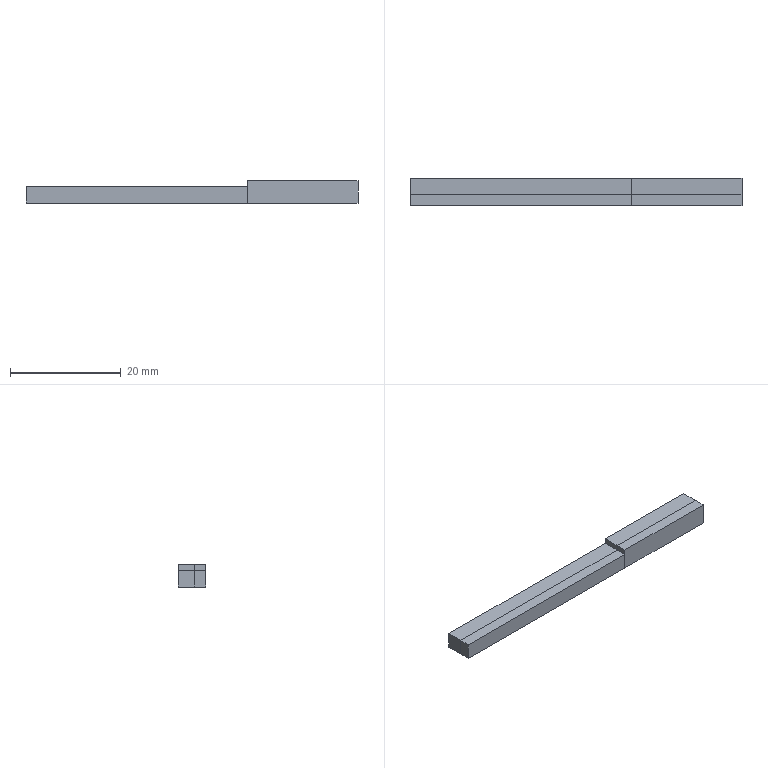Part | SolidWorks | features ICE 3, Extrusion 1 | 4 solids | 24 faces | box 60 x 5 x 4 mm | volume 1000 mm3 | plane 24
STEP:
#1=CARTESIAN_POINT('',(-10.,0.,-2.));
#2=VERTEX_POINT('',#1);
#3=CARTESIAN_POINT('',(-10.,0.,2.));
#4=VERTEX_POINT('',#3);
#5=CARTESIAN_POINT('',(-10.,0.,2.));
#6=DIRECTION('',(0.,0.,1.));
#7=VECTOR('',#6,1000.);
#8=LINE('',#5,#7);
#9=EDGE_CURVE('',#2,#4,#8,.T.);
#10=ORIENTED_EDGE('',*,*,#9,.T.);
#11=CARTESIAN_POINT('',(-10.,2.,2.));
#12=VERTEX_POINT('',#11);
#13=CARTESIAN_POINT('',(-10.,2.,2.));
#14=DIRECTION('',(0.,-1.,0.));
#15=VECTOR('',#14,1000.);
#16=LINE('',#13,#15);
#17=EDGE_CURVE('',#12,#4,#16,.T.);
#18=ORIENTED_EDGE('',*,*,#17,.F.);
#19=CARTESIAN_POINT('',(-10.,2.,-2.));
#20=VERTEX_POINT('',#19);
#21=CARTESIAN_POINT('',(-10.,2.,2.));
#22=DIRECTION('',(0.,0.,1.));
#23=VECTOR('',#22,1000.);
#24=LINE('',#21,#23);
#25=EDGE_CURVE('',#20,#12,#24,.T.);
#26=ORIENTED_EDGE('',*,*,#25,.F.);
#27=CARTESIAN_POINT('',(-10.,2.,-2.));
#28=DIRECTION('',(0.,-1.,0.));
#29=VECTOR('',#28,1000.);
#30=LINE('',#27,#29);
#31=EDGE_CURVE('',#20,#2,#30,.T.);
#32=ORIENTED_EDGE('',*,*,#31,.T.);
#33=EDGE_LOOP('',(#10,#18,#26,#32));
#34=FACE_OUTER_BOUND('',#33,.T.);
#35=CARTESIAN_POINT('',(-10.,2.,2.));
#36=DIRECTION('',(1.,0.,0.));
#37=DIRECTION('',(0.,0.,-1.));
#38=AXIS2_PLACEMENT_3D('',#35,#36,#37);
#39=PLANE('',#38);
#40=ADVANCED_FACE('',(#34),#39,.F.);
#41=CARTESIAN_POINT('',(10.,0.,2.));
#42=VERTEX_POINT('',#41);
#43=CARTESIAN_POINT('',(10.,0.,2.));
#44=DIRECTION('',(1.,0.,0.));
#45=VECTOR('',#44,1000.);
#46=LINE('',#43,#45);
#47=EDGE_CURVE('',#4,#42,#46,.T.);
#48=ORIENTED_EDGE('',*,*,#47,.T.);
#49=CARTESIAN_POINT('',(10.,2.,2.));
#50=VERTEX_POINT('',#49);
#51=CARTESIAN_POINT('',(10.,2.,2.));
#52=DIRECTION('',(0.,-1.,0.));
#53=VECTOR('',#52,1000.);
#54=LINE('',#51,#53);
#55=EDGE_CURVE('',#50,#42,#54,.T.);
#56=ORIENTED_EDGE('',*,*,#55,.F.);
#57=CARTESIAN_POINT('',(10.,2.,2.));
#58=DIRECTION('',(1.,0.,0.));
#59=VECTOR('',#58,1000.);
#60=LINE('',#57,#59);
#61=EDGE_CURVE('',#12,#50,#60,.T.);
#62=ORIENTED_EDGE('',*,*,#61,.F.);
#63=ORIENTED_EDGE('',*,*,#17,.T.);
#64=EDGE_LOOP('',(#48,#56,#62,#63));
#65=FACE_OUTER_BOUND('',#64,.T.);
#66=CARTESIAN_POINT('',(10.,2.,2.));
#67=DIRECTION('',(0.,0.,-1.));
#68=DIRECTION('',(-1.,0.,0.));
#69=AXIS2_PLACEMENT_3D('',#66,#67,#68);
#70=PLANE('',#69);
#71=ADVANCED_FACE('',(#65),#70,.F.);
#72=CARTESIAN_POINT('',(10.,0.,-2.));
#73=VERTEX_POINT('',#72);
#74=CARTESIAN_POINT('',(10.,0.,2.));
#75=DIRECTION('',(0.,0.,-1.));
#76=VECTOR('',#75,1000.);
#77=LINE('',#74,#76);
#78=EDGE_CURVE('',#42,#73,#77,.T.);
#79=ORIENTED_EDGE('',*,*,#78,.T.);
#80=CARTESIAN_POINT('',(10.,2.,-2.));
#81=VERTEX_POINT('',#80);
#82=CARTESIAN_POINT('',(10.,2.,-2.));
#83=DIRECTION('',(0.,-1.,0.));
#84=VECTOR('',#83,1000.);
#85=LINE('',#82,#84);
#86=EDGE_CURVE('',#81,#73,#85,.T.);
#87=ORIENTED_EDGE('',*,*,#86,.F.);
#88=CARTESIAN_POINT('',(10.,2.,2.));
#89=DIRECTION('',(0.,0.,-1.));
#90=VECTOR('',#89,1000.);
#91=LINE('',#88,#90);
#92=EDGE_CURVE('',#50,#81,#91,.T.);
#93=ORIENTED_EDGE('',*,*,#92,.F.);
#94=ORIENTED_EDGE('',*,*,#55,.T.);
#95=EDGE_LOOP('',(#79,#87,#93,#94));
#96=FACE_OUTER_BOUND('',#95,.T.);
#97=CARTESIAN_POINT('',(10.,2.,2.));
#98=DIRECTION('',(-1.,0.,0.));
#99=DIRECTION('',(0.,0.,1.));
#100=AXIS2_PLACEMENT_3D('',#97,#98,#99);
#101=PLANE('',#100);
#102=ADVANCED_FACE('',(#96),#101,.F.);
#103=CARTESIAN_POINT('',(10.,0.,-2.));
#104=DIRECTION('',(-1.,0.,0.));
#105=VECTOR('',#104,1000.);
#106=LINE('',#103,#105);
#107=EDGE_CURVE('',#73,#2,#106,.T.);
#108=ORIENTED_EDGE('',*,*,#107,.T.);
#109=ORIENTED_EDGE('',*,*,#31,.F.);
#110=CARTESIAN_POINT('',(10.,2.,-2.));
#111=DIRECTION('',(-1.,0.,0.));
#112=VECTOR('',#111,1000.);
#113=LINE('',#110,#112);
#114=EDGE_CURVE('',#81,#20,#113,.T.);
#115=ORIENTED_EDGE('',*,*,#114,.F.);
#116=ORIENTED_EDGE('',*,*,#86,.T.);
#117=EDGE_LOOP('',(#108,#109,#115,#116));
#118=FACE_OUTER_BOUND('',#117,.T.);
#119=CARTESIAN_POINT('',(10.,2.,-2.));
#120=DIRECTION('',(0.,0.,1.));
#121=DIRECTION('',(1.,0.,0.));
#122=AXIS2_PLACEMENT_3D('',#119,#120,#121);
#123=PLANE('',#122);
#124=ADVANCED_FACE('',(#118),#123,.F.);
#125=ORIENTED_EDGE('',*,*,#25,.T.);
#126=ORIENTED_EDGE('',*,*,#61,.T.);
#127=ORIENTED_EDGE('',*,*,#92,.T.);
#128=ORIENTED_EDGE('',*,*,#114,.T.);
#129=EDGE_LOOP('',(#125,#126,#127,#128));
#130=FACE_OUTER_BOUND('',#129,.T.);
#131=CARTESIAN_POINT('',(0.,2.,0.));
#132=DIRECTION('',(0.,1.,0.));
#133=DIRECTION('',(0.,0.,1.));
#134=AXIS2_PLACEMENT_3D('',#131,#132,#133);
#135=PLANE('',#134);
#136=ADVANCED_FACE('',(#130),#135,.T.);
#137=ORIENTED_EDGE('',*,*,#9,.F.);
#138=ORIENTED_EDGE('',*,*,#107,.F.);
#139=ORIENTED_EDGE('',*,*,#78,.F.);
#140=ORIENTED_EDGE('',*,*,#47,.F.);
#141=EDGE_LOOP('',(#137,#138,#139,#140));
#142=FACE_OUTER_BOUND('',#141,.T.);
#143=CARTESIAN_POINT('',(0.,0.,0.));
#144=DIRECTION('',(0.,1.,0.));
#145=DIRECTION('',(0.,0.,1.));
#146=AXIS2_PLACEMENT_3D('',#143,#144,#145);
#147=PLANE('',#146);
#148=ADVANCED_FACE('',(#142),#147,.F.);
#149=CLOSED_SHELL('',(#40,#71,#102,#124,#136,#148));
#150=MANIFOLD_SOLID_BREP('',#149);
#151=CARTESIAN_POINT('',(10.,2.,-2.));
#152=VERTEX_POINT('',#151);
#153=CARTESIAN_POINT('',(-10.,2.,-2.));
#154=VERTEX_POINT('',#153);
#155=CARTESIAN_POINT('',(10.,2.,-2.));
#156=DIRECTION('',(-1.,0.,0.));
#157=VECTOR('',#156,1000.);
#158=LINE('',#155,#157);
#159=EDGE_CURVE('',#152,#154,#158,.T.);
#160=ORIENTED_EDGE('',*,*,#159,.T.);
#161=CARTESIAN_POINT('',(-10.,5.,-2.));
#162=VERTEX_POINT('',#161);
#163=CARTESIAN_POINT('',(-10.,5.,-2.));
#164=DIRECTION('',(0.,-1.,0.));
#165=VECTOR('',#164,1000.);
#166=LINE('',#163,#165);
#167=EDGE_CURVE('',#162,#154,#166,.T.);
#168=ORIENTED_EDGE('',*,*,#167,.F.);
#169=CARTESIAN_POINT('',(10.,5.,-2.));
#170=VERTEX_POINT('',#169);
#171=CARTESIAN_POINT('',(10.,5.,-2.));
#172=DIRECTION('',(-1.,0.,0.));
#173=VECTOR('',#172,1000.);
#174=LINE('',#171,#173);
#175=EDGE_CURVE('',#170,#162,#174,.T.);
#176=ORIENTED_EDGE('',*,*,#175,.F.);
#177=CARTESIAN_POINT('',(10.,5.,-2.));
#178=DIRECTION('',(0.,-1.,0.));
#179=VECTOR('',#178,1000.);
#180=LINE('',#177,#179);
#181=EDGE_CURVE('',#170,#152,#180,.T.);
#182=ORIENTED_EDGE('',*,*,#181,.T.);
#183=EDGE_LOOP('',(#160,#168,#176,#182));
#184=FACE_OUTER_BOUND('',#183,.T.);
#185=CARTESIAN_POINT('',(10.,5.,-2.));
#186=DIRECTION('',(0.,0.,1.));
#187=DIRECTION('',(1.,0.,0.));
#188=AXIS2_PLACEMENT_3D('',#185,#186,#187);
#189=PLANE('',#188);
#190=ADVANCED_FACE('',(#184),#189,.F.);
#191=CARTESIAN_POINT('',(-10.,2.,2.));
#192=VERTEX_POINT('',#191);
#193=CARTESIAN_POINT('',(-10.,2.,-2.));
#194=DIRECTION('',(0.,0.,1.));
#195=VECTOR('',#194,1000.);
#196=LINE('',#193,#195);
#197=EDGE_CURVE('',#154,#192,#196,.T.);
#198=ORIENTED_EDGE('',*,*,#197,.T.);
#199=CARTESIAN_POINT('',(-10.,5.,2.));
#200=VERTEX_POINT('',#199);
#201=CARTESIAN_POINT('',(-10.,5.,2.));
#202=DIRECTION('',(0.,-1.,0.));
#203=VECTOR('',#202,1000.);
#204=LINE('',#201,#203);
#205=EDGE_CURVE('',#200,#192,#204,.T.);
#206=ORIENTED_EDGE('',*,*,#205,.F.);
#207=CARTESIAN_POINT('',(-10.,5.,-2.));
#208=DIRECTION('',(0.,0.,1.));
#209=VECTOR('',#208,1000.);
#210=LINE('',#207,#209);
#211=EDGE_CURVE('',#162,#200,#210,.T.);
#212=ORIENTED_EDGE('',*,*,#211,.F.);
#213=ORIENTED_EDGE('',*,*,#167,.T.);
#214=EDGE_LOOP('',(#198,#206,#212,#213));
#215=FACE_OUTER_BOUND('',#214,.T.);
#216=CARTESIAN_POINT('',(-10.,5.,-2.));
#217=DIRECTION('',(1.,0.,0.));
#218=DIRECTION('',(0.,0.,-1.));
#219=AXIS2_PLACEMENT_3D('',#216,#217,#218);
#220=PLANE('',#219);
#221=ADVANCED_FACE('',(#215),#220,.F.);
#222=CARTESIAN_POINT('',(10.,2.,2.));
#223=VERTEX_POINT('',#222);
#224=CARTESIAN_POINT('',(-10.,2.,2.));
#225=DIRECTION('',(1.,0.,0.));
#226=VECTOR('',#225,1000.);
#227=LINE('',#224,#226);
#228=EDGE_CURVE('',#192,#223,#227,.T.);
#229=ORIENTED_EDGE('',*,*,#228,.T.);
#230=CARTESIAN_POINT('',(10.,5.,2.));
#231=VERTEX_POINT('',#230);
#232=CARTESIAN_POINT('',(10.,5.,2.));
#233=DIRECTION('',(0.,-1.,0.));
#234=VECTOR('',#233,1000.);
#235=LINE('',#232,#234);
#236=EDGE_CURVE('',#231,#223,#235,.T.);
#237=ORIENTED_EDGE('',*,*,#236,.F.);
#238=CARTESIAN_POINT('',(-10.,5.,2.));
#239=DIRECTION('',(1.,0.,0.));
#240=VECTOR('',#239,1000.);
#241=LINE('',#238,#240);
#242=EDGE_CURVE('',#200,#231,#241,.T.);
#243=ORIENTED_EDGE('',*,*,#242,.F.);
#244=ORIENTED_EDGE('',*,*,#205,.T.);
#245=EDGE_LOOP('',(#229,#237,#243,#244));
#246=FACE_OUTER_BOUND('',#245,.T.);
#247=CARTESIAN_POINT('',(-10.,5.,2.));
#248=DIRECTION('',(0.,0.,-1.));
#249=DIRECTION('',(-1.,0.,0.));
#250=AXIS2_PLACEMENT_3D('',#247,#248,#249);
#251=PLANE('',#250);
#252=ADVANCED_FACE('',(#246),#251,.F.);
#253=CARTESIAN_POINT('',(10.,2.,2.));
#254=DIRECTION('',(0.,0.,-1.));
#255=VECTOR('',#254,1000.);
#256=LINE('',#253,#255);
#257=EDGE_CURVE('',#223,#152,#256,.T.);
#258=ORIENTED_EDGE('',*,*,#257,.T.);
#259=ORIENTED_EDGE('',*,*,#181,.F.);
#260=CARTESIAN_POINT('',(10.,5.,2.));
#261=DIRECTION('',(0.,0.,-1.));
#262=VECTOR('',#261,1000.);
#263=LINE('',#260,#262);
#264=EDGE_CURVE('',#231,#170,#263,.T.);
#265=ORIENTED_EDGE('',*,*,#264,.F.);
#266=ORIENTED_EDGE('',*,*,#236,.T.);
#267=EDGE_LOOP('',(#258,#259,#265,#266));
#268=FACE_OUTER_BOUND('',#267,.T.);
#269=CARTESIAN_POINT('',(10.,5.,2.));
#270=DIRECTION('',(-1.,0.,0.));
#271=DIRECTION('',(0.,0.,1.));
#272=AXIS2_PLACEMENT_3D('',#269,#270,#271);
#273=PLANE('',#272);
#274=ADVANCED_FACE('',(#268),#273,.F.);
#275=ORIENTED_EDGE('',*,*,#175,.T.);
#276=ORIENTED_EDGE('',*,*,#211,.T.);
#277=ORIENTED_EDGE('',*,*,#242,.T.);
#278=ORIENTED_EDGE('',*,*,#264,.T.);
#279=EDGE_LOOP('',(#275,#276,#277,#278));
#280=FACE_OUTER_BOUND('',#279,.T.);
#281=CARTESIAN_POINT('',(0.,5.,0.));
#282=DIRECTION('',(0.,1.,0.));
#283=DIRECTION('',(0.,0.,1.));
#284=AXIS2_PLACEMENT_3D('',#281,#282,#283);
#285=PLANE('',#284);
#286=ADVANCED_FACE('',(#280),#285,.T.);
#287=ORIENTED_EDGE('',*,*,#159,.F.);
#288=ORIENTED_EDGE('',*,*,#257,.F.);
#289=ORIENTED_EDGE('',*,*,#228,.F.);
#290=ORIENTED_EDGE('',*,*,#197,.F.);
#291=EDGE_LOOP('',(#287,#288,#289,#290));
#292=FACE_OUTER_BOUND('',#291,.T.);
#293=CARTESIAN_POINT('',(0.,2.,0.));
#294=DIRECTION('',(0.,1.,0.));
#295=DIRECTION('',(0.,0.,1.));
#296=AXIS2_PLACEMENT_3D('',#293,#294,#295);
#297=PLANE('',#296);
#298=ADVANCED_FACE('',(#292),#297,.F.);
#299=CLOSED_SHELL('',(#190,#221,#252,#274,#286,#298));
#300=MANIFOLD_SOLID_BREP('',#299);
#301=CARTESIAN_POINT('',(-10.,0.,-2.));
#302=VERTEX_POINT('',#301);
#303=CARTESIAN_POINT('',(-10.,0.,1.));
#304=VERTEX_POINT('',#303);
#305=CARTESIAN_POINT('',(-10.,0.,1.));
#306=DIRECTION('',(0.,0.,1.));
#307=VECTOR('',#306,1000.);
#308=LINE('',#305,#307);
#309=EDGE_CURVE('',#302,#304,#308,.T.);
#310=ORIENTED_EDGE('',*,*,#309,.F.);
#311=CARTESIAN_POINT('',(-10.,2.,-2.));
#312=VERTEX_POINT('',#311);
#313=CARTESIAN_POINT('',(-10.,2.,-2.));
#314=DIRECTION('',(0.,-1.,0.));
#315=VECTOR('',#314,1000.);
#316=LINE('',#313,#315);
#317=EDGE_CURVE('',#312,#302,#316,.T.);
#318=ORIENTED_EDGE('',*,*,#317,.F.);
#319=CARTESIAN_POINT('',(-10.,2.,1.));
#320=VERTEX_POINT('',#319);
#321=CARTESIAN_POINT('',(-10.,2.,1.));
#322=DIRECTION('',(0.,0.,1.));
#323=VECTOR('',#322,1000.);
#324=LINE('',#321,#323);
#325=EDGE_CURVE('',#312,#320,#324,.T.);
#326=ORIENTED_EDGE('',*,*,#325,.T.);
#327=CARTESIAN_POINT('',(-10.,2.,1.));
#328=DIRECTION('',(0.,-1.,0.));
#329=VECTOR('',#328,1000.);
#330=LINE('',#327,#329);
#331=EDGE_CURVE('',#320,#304,#330,.T.);
#332=ORIENTED_EDGE('',*,*,#331,.T.);
#333=EDGE_LOOP('',(#310,#318,#326,#332));
#334=FACE_OUTER_BOUND('',#333,.T.);
#335=CARTESIAN_POINT('',(-10.,2.,1.));
#336=DIRECTION('',(1.,0.,0.));
#337=DIRECTION('',(0.,0.,-1.));
#338=AXIS2_PLACEMENT_3D('',#335,#336,#337);
#339=PLANE('',#338);
#340=ADVANCED_FACE('',(#334),#339,.T.);
#341=CARTESIAN_POINT('',(-50.,0.,-2.));
#342=VERTEX_POINT('',#341);
#343=CARTESIAN_POINT('',(-10.,0.,-2.));
#344=DIRECTION('',(1.,0.,0.));
#345=VECTOR('',#344,1000.);
#346=LINE('',#343,#345);
#347=EDGE_CURVE('',#342,#302,#346,.T.);
#348=ORIENTED_EDGE('',*,*,#347,.F.);
#349=CARTESIAN_POINT('',(-50.,2.,-2.));
#350=VERTEX_POINT('',#349);
#351=CARTESIAN_POINT('',(-50.,2.,-2.));
#352=DIRECTION('',(0.,-1.,0.));
#353=VECTOR('',#352,1000.);
#354=LINE('',#351,#353);
#355=EDGE_CURVE('',#350,#342,#354,.T.);
#356=ORIENTED_EDGE('',*,*,#355,.F.);
#357=CARTESIAN_POINT('',(-10.,2.,-2.));
#358=DIRECTION('',(1.,0.,0.));
#359=VECTOR('',#358,1000.);
#360=LINE('',#357,#359);
#361=EDGE_CURVE('',#350,#312,#360,.T.);
#362=ORIENTED_EDGE('',*,*,#361,.T.);
#363=ORIENTED_EDGE('',*,*,#317,.T.);
#364=EDGE_LOOP('',(#348,#356,#362,#363));
#365=FACE_OUTER_BOUND('',#364,.T.);
#366=CARTESIAN_POINT('',(-10.,2.,-2.));
#367=DIRECTION('',(0.,0.,-1.));
#368=DIRECTION('',(-1.,0.,0.));
#369=AXIS2_PLACEMENT_3D('',#366,#367,#368);
#370=PLANE('',#369);
#371=ADVANCED_FACE('',(#365),#370,.T.);
#372=CARTESIAN_POINT('',(-50.,0.,1.));
#373=VERTEX_POINT('',#372);
#374=CARTESIAN_POINT('',(-50.,0.,1.));
#375=DIRECTION('',(0.,0.,-1.));
#376=VECTOR('',#375,1000.);
#377=LINE('',#374,#376);
#378=EDGE_CURVE('',#373,#342,#377,.T.);
#379=ORIENTED_EDGE('',*,*,#378,.F.);
#380=CARTESIAN_POINT('',(-50.,2.,1.));
#381=VERTEX_POINT('',#380);
#382=CARTESIAN_POINT('',(-50.,2.,1.));
#383=DIRECTION('',(0.,-1.,0.));
#384=VECTOR('',#383,1000.);
#385=LINE('',#382,#384);
#386=EDGE_CURVE('',#381,#373,#385,.T.);
#387=ORIENTED_EDGE('',*,*,#386,.F.);
#388=CARTESIAN_POINT('',(-50.,2.,1.));
#389=DIRECTION('',(0.,0.,-1.));
#390=VECTOR('',#389,1000.);
#391=LINE('',#388,#390);
#392=EDGE_CURVE('',#381,#350,#391,.T.);
#393=ORIENTED_EDGE('',*,*,#392,.T.);
#394=ORIENTED_EDGE('',*,*,#355,.T.);
#395=EDGE_LOOP('',(#379,#387,#393,#394));
#396=FACE_OUTER_BOUND('',#395,.T.);
#397=CARTESIAN_POINT('',(-50.,2.,1.));
#398=DIRECTION('',(-1.,0.,0.));
#399=DIRECTION('',(0.,0.,1.));
#400=AXIS2_PLACEMENT_3D('',#397,#398,#399);
#401=PLANE('',#400);
#402=ADVANCED_FACE('',(#396),#401,.T.);
#403=CARTESIAN_POINT('',(-10.,0.,1.));
#404=DIRECTION('',(-1.,0.,0.));
#405=VECTOR('',#404,1000.);
#406=LINE('',#403,#405);
#407=EDGE_CURVE('',#304,#373,#406,.T.);
#408=ORIENTED_EDGE('',*,*,#407,.F.);
#409=ORIENTED_EDGE('',*,*,#331,.F.);
#410=CARTESIAN_POINT('',(-10.,2.,1.));
#411=DIRECTION('',(-1.,0.,0.));
#412=VECTOR('',#411,1000.);
#413=LINE('',#410,#412);
#414=EDGE_CURVE('',#320,#381,#413,.T.);
#415=ORIENTED_EDGE('',*,*,#414,.T.);
#416=ORIENTED_EDGE('',*,*,#386,.T.);
#417=EDGE_LOOP('',(#408,#409,#415,#416));
#418=FACE_OUTER_BOUND('',#417,.T.);
#419=CARTESIAN_POINT('',(-10.,2.,1.));
#420=DIRECTION('',(0.,0.,1.));
#421=DIRECTION('',(1.,0.,0.));
#422=AXIS2_PLACEMENT_3D('',#419,#420,#421);
#423=PLANE('',#422);
#424=ADVANCED_FACE('',(#418),#423,.T.);
#425=ORIENTED_EDGE('',*,*,#325,.F.);
#426=ORIENTED_EDGE('',*,*,#361,.F.);
#427=ORIENTED_EDGE('',*,*,#392,.F.);
#428=ORIENTED_EDGE('',*,*,#414,.F.);
#429=EDGE_LOOP('',(#425,#426,#427,#428));
#430=FACE_OUTER_BOUND('',#429,.T.);
#431=CARTESIAN_POINT('',(0.,2.,0.));
#432=DIRECTION('',(0.,1.,0.));
#433=DIRECTION('',(0.,0.,1.));
#434=AXIS2_PLACEMENT_3D('',#431,#432,#433);
#435=PLANE('',#434);
#436=ADVANCED_FACE('',(#430),#435,.T.);
#437=ORIENTED_EDGE('',*,*,#309,.T.);
#438=ORIENTED_EDGE('',*,*,#407,.T.);
#439=ORIENTED_EDGE('',*,*,#378,.T.);
#440=ORIENTED_EDGE('',*,*,#347,.T.);
#441=EDGE_LOOP('',(#437,#438,#439,#440));
#442=FACE_OUTER_BOUND('',#441,.T.);
#443=CARTESIAN_POINT('',(0.,0.,0.));
#444=DIRECTION('',(0.,1.,0.));
#445=DIRECTION('',(0.,0.,1.));
#446=AXIS2_PLACEMENT_3D('',#443,#444,#445);
#447=PLANE('',#446);
#448=ADVANCED_FACE('',(#442),#447,.F.);
#449=CLOSED_SHELL('',(#340,#371,#402,#424,#436,#448));
#450=MANIFOLD_SOLID_BREP('',#449);
#451=CARTESIAN_POINT('',(-50.,2.,-2.));
#452=VERTEX_POINT('',#451);
#453=CARTESIAN_POINT('',(-50.,2.,1.));
#454=VERTEX_POINT('',#453);
#455=CARTESIAN_POINT('',(-50.,2.,-2.));
#456=DIRECTION('',(0.,0.,1.));
#457=VECTOR('',#456,1000.);
#458=LINE('',#455,#457);
#459=EDGE_CURVE('',#452,#454,#458,.T.);
#460=ORIENTED_EDGE('',*,*,#459,.T.);
#461=CARTESIAN_POINT('',(-50.,5.,1.));
#462=VERTEX_POINT('',#461);
#463=CARTESIAN_POINT('',(-50.,5.,1.));
#464=DIRECTION('',(0.,-1.,0.));
#465=VECTOR('',#464,1000.);
#466=LINE('',#463,#465);
#467=EDGE_CURVE('',#462,#454,#466,.T.);
#468=ORIENTED_EDGE('',*,*,#467,.F.);
#469=CARTESIAN_POINT('',(-50.,5.,-2.));
#470=VERTEX_POINT('',#469);
#471=CARTESIAN_POINT('',(-50.,5.,-2.));
#472=DIRECTION('',(0.,0.,1.));
#473=VECTOR('',#472,1000.);
#474=LINE('',#471,#473);
#475=EDGE_CURVE('',#470,#462,#474,.T.);
#476=ORIENTED_EDGE('',*,*,#475,.F.);
#477=CARTESIAN_POINT('',(-50.,5.,-2.));
#478=DIRECTION('',(0.,-1.,0.));
#479=VECTOR('',#478,1000.);
#480=LINE('',#477,#479);
#481=EDGE_CURVE('',#470,#452,#480,.T.);
#482=ORIENTED_EDGE('',*,*,#481,.T.);
#483=EDGE_LOOP('',(#460,#468,#476,#482));
#484=FACE_OUTER_BOUND('',#483,.T.);
#485=CARTESIAN_POINT('',(-50.,5.,-2.));
#486=DIRECTION('',(1.,0.,0.));
#487=DIRECTION('',(0.,0.,-1.));
#488=AXIS2_PLACEMENT_3D('',#485,#486,#487);
#489=PLANE('',#488);
#490=ADVANCED_FACE('',(#484),#489,.F.);
#491=CARTESIAN_POINT('',(-10.,2.,1.));
#492=VERTEX_POINT('',#491);
#493=CARTESIAN_POINT('',(-50.,2.,1.));
#494=DIRECTION('',(1.,0.,0.));
#495=VECTOR('',#494,1000.);
#496=LINE('',#493,#495);
#497=EDGE_CURVE('',#454,#492,#496,.T.);
#498=ORIENTED_EDGE('',*,*,#497,.T.);
#499=CARTESIAN_POINT('',(-10.,5.,1.));
#500=VERTEX_POINT('',#499);
#501=CARTESIAN_POINT('',(-10.,5.,1.));
#502=DIRECTION('',(0.,-1.,0.));
#503=VECTOR('',#502,1000.);
#504=LINE('',#501,#503);
#505=EDGE_CURVE('',#500,#492,#504,.T.);
#506=ORIENTED_EDGE('',*,*,#505,.F.);
#507=CARTESIAN_POINT('',(-50.,5.,1.));
#508=DIRECTION('',(1.,0.,0.));
#509=VECTOR('',#508,1000.);
#510=LINE('',#507,#509);
#511=EDGE_CURVE('',#462,#500,#510,.T.);
#512=ORIENTED_EDGE('',*,*,#511,.F.);
#513=ORIENTED_EDGE('',*,*,#467,.T.);
#514=EDGE_LOOP('',(#498,#506,#512,#513));
#515=FACE_OUTER_BOUND('',#514,.T.);
#516=CARTESIAN_POINT('',(-50.,5.,1.));
#517=DIRECTION('',(0.,0.,-1.));
#518=DIRECTION('',(-1.,0.,0.));
#519=AXIS2_PLACEMENT_3D('',#516,#517,#518);
#520=PLANE('',#519);
#521=ADVANCED_FACE('',(#515),#520,.F.);
#522=CARTESIAN_POINT('',(-10.,2.,-2.));
#523=VERTEX_POINT('',#522);
#524=CARTESIAN_POINT('',(-10.,2.,-2.));
#525=DIRECTION('',(0.,0.,-1.));
#526=VECTOR('',#525,1000.);
#527=LINE('',#524,#526);
#528=EDGE_CURVE('',#492,#523,#527,.T.);
#529=ORIENTED_EDGE('',*,*,#528,.T.);
#530=CARTESIAN_POINT('',(-10.,5.,-2.));
#531=VERTEX_POINT('',#530);
#532=CARTESIAN_POINT('',(-10.,5.,-2.));
#533=DIRECTION('',(0.,-1.,0.));
#534=VECTOR('',#533,1000.);
#535=LINE('',#532,#534);
#536=EDGE_CURVE('',#531,#523,#535,.T.);
#537=ORIENTED_EDGE('',*,*,#536,.F.);
#538=CARTESIAN_POINT('',(-10.,5.,-2.));
#539=DIRECTION('',(0.,0.,-1.));
#540=VECTOR('',#539,1000.);
#541=LINE('',#538,#540);
#542=EDGE_CURVE('',#500,#531,#541,.T.);
#543=ORIENTED_EDGE('',*,*,#542,.F.);
#544=ORIENTED_EDGE('',*,*,#505,.T.);
#545=EDGE_LOOP('',(#529,#537,#543,#544));
#546=FACE_OUTER_BOUND('',#545,.T.);
#547=CARTESIAN_POINT('',(-10.,5.,-2.));
#548=DIRECTION('',(-1.,0.,0.));
#549=DIRECTION('',(0.,0.,1.));
#550=AXIS2_PLACEMENT_3D('',#547,#548,#549);
#551=PLANE('',#550);
#552=ADVANCED_FACE('',(#546),#551,.F.);
#553=CARTESIAN_POINT('',(-50.,2.,-2.));
#554=DIRECTION('',(-1.,0.,0.));
#555=VECTOR('',#554,1000.);
#556=LINE('',#553,#555);
#557=EDGE_CURVE('',#523,#452,#556,.T.);
#558=ORIENTED_EDGE('',*,*,#557,.T.);
#559=ORIENTED_EDGE('',*,*,#481,.F.);
#560=CARTESIAN_POINT('',(-50.,5.,-2.));
#561=DIRECTION('',(-1.,0.,0.));
#562=VECTOR('',#561,1000.);
#563=LINE('',#560,#562);
#564=EDGE_CURVE('',#531,#470,#563,.T.);
#565=ORIENTED_EDGE('',*,*,#564,.F.);
#566=ORIENTED_EDGE('',*,*,#536,.T.);
#567=EDGE_LOOP('',(#558,#559,#565,#566));
#568=FACE_OUTER_BOUND('',#567,.T.);
#569=CARTESIAN_POINT('',(-50.,5.,-2.));
#570=DIRECTION('',(0.,0.,1.));
#571=DIRECTION('',(1.,0.,0.));
#572=AXIS2_PLACEMENT_3D('',#569,#570,#571);
#573=PLANE('',#572);
#574=ADVANCED_FACE('',(#568),#573,.F.);
#575=ORIENTED_EDGE('',*,*,#475,.T.);
#576=ORIENTED_EDGE('',*,*,#511,.T.);
#577=ORIENTED_EDGE('',*,*,#542,.T.);
#578=ORIENTED_EDGE('',*,*,#564,.T.);
#579=EDGE_LOOP('',(#575,#576,#577,#578));
#580=FACE_OUTER_BOUND('',#579,.T.);
#581=CARTESIAN_POINT('',(0.,5.,0.));
#582=DIRECTION('',(0.,1.,0.));
#583=DIRECTION('',(0.,0.,1.));
#584=AXIS2_PLACEMENT_3D('',#581,#582,#583);
#585=PLANE('',#584);
#586=ADVANCED_FACE('',(#580),#585,.T.);
#587=ORIENTED_EDGE('',*,*,#459,.F.);
#588=ORIENTED_EDGE('',*,*,#557,.F.);
#589=ORIENTED_EDGE('',*,*,#528,.F.);
#590=ORIENTED_EDGE('',*,*,#497,.F.);
#591=EDGE_LOOP('',(#587,#588,#589,#590));
#592=FACE_OUTER_BOUND('',#591,.T.);
#593=CARTESIAN_POINT('',(0.,2.,0.));
#594=DIRECTION('',(0.,1.,0.));
#595=DIRECTION('',(0.,0.,1.));
#596=AXIS2_PLACEMENT_3D('',#593,#594,#595);
#597=PLANE('',#596);
#598=ADVANCED_FACE('',(#592),#597,.F.);
#599=CLOSED_SHELL('',(#490,#521,#552,#574,#586,#598));
#600=MANIFOLD_SOLID_BREP('',#599);
#601=CARTESIAN_POINT('',(0.,0.,0.));
#602=DIRECTION('',(0.,0.,1.));
#603=DIRECTION('',(1.,0.,0.));
#604=AXIS2_PLACEMENT_3D('',#601,#602,#603);
#605=(LENGTH_UNIT()NAMED_UNIT(*)SI_UNIT(.MILLI.,.METRE.));
#606=UNCERTAINTY_MEASURE_WITH_UNIT(LENGTH_MEASURE(0.00001),#605,'','');
#607=(NAMED_UNIT(*)PLANE_ANGLE_UNIT()SI_UNIT($,.RADIAN.));
#608=(NAMED_UNIT(*)SI_UNIT($,.STERADIAN.)SOLID_ANGLE_UNIT());
#609=(GEOMETRIC_REPRESENTATION_CONTEXT(3)GLOBAL_UNCERTAINTY_ASSIGNED_CONTEXT((#606))GLOBAL_UNIT_ASSIGNED_CONTEXT((#605,#607,#608))REPRESENTATION_CONTEXT('',''));
#610=ADVANCED_BREP_SHAPE_REPRESENTATION('',(#150,#300,#450,#600,#604),#609);